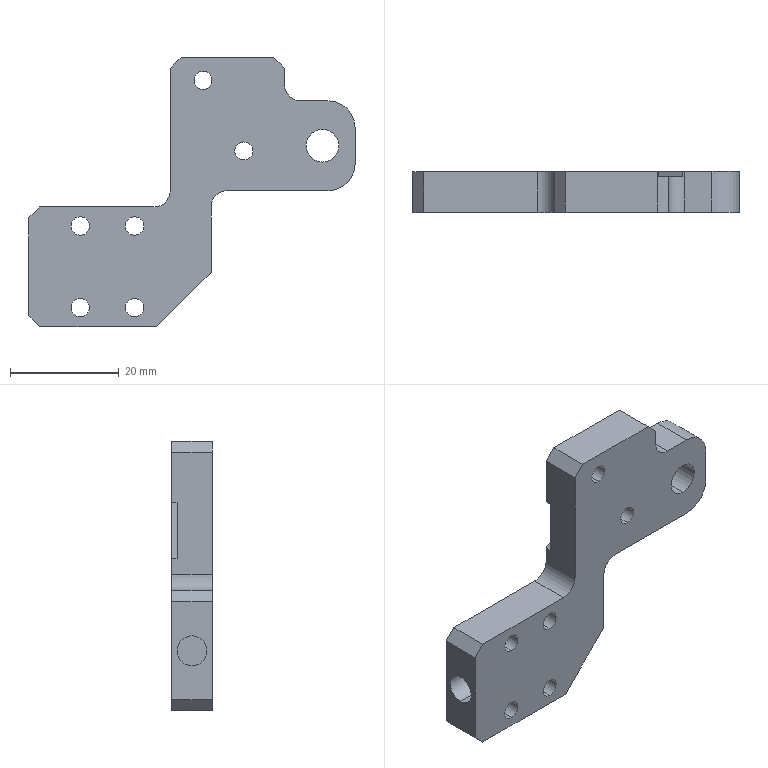Part | SolidWorks | features HoleWzd 3, ICE 3, Chamfer 2, Fillet 2, Extrusion 1 | 1 solid | 55 faces | box 60 x 7.5 x 49.5 mm | volume 9409 mm3 | cylinder 29 | plane 26 | commonest cylinder face diameters 6 x13 3.4 x8 3.3 x4 5.5 x2 10 x2